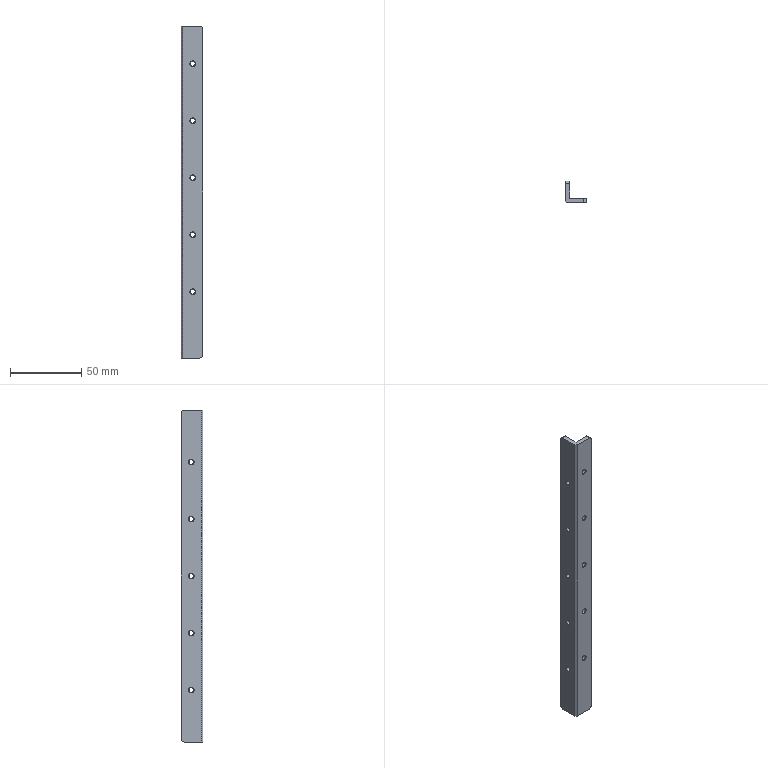Part | STEP file | SOLID | 1 solid | 33 faces | box 15 x 15 x 233 mm | volume 18483 mm3 | cylinder 14 | cone 10 | plane 9 | commonest cylinder face diameters 3.3 x10 4 x4